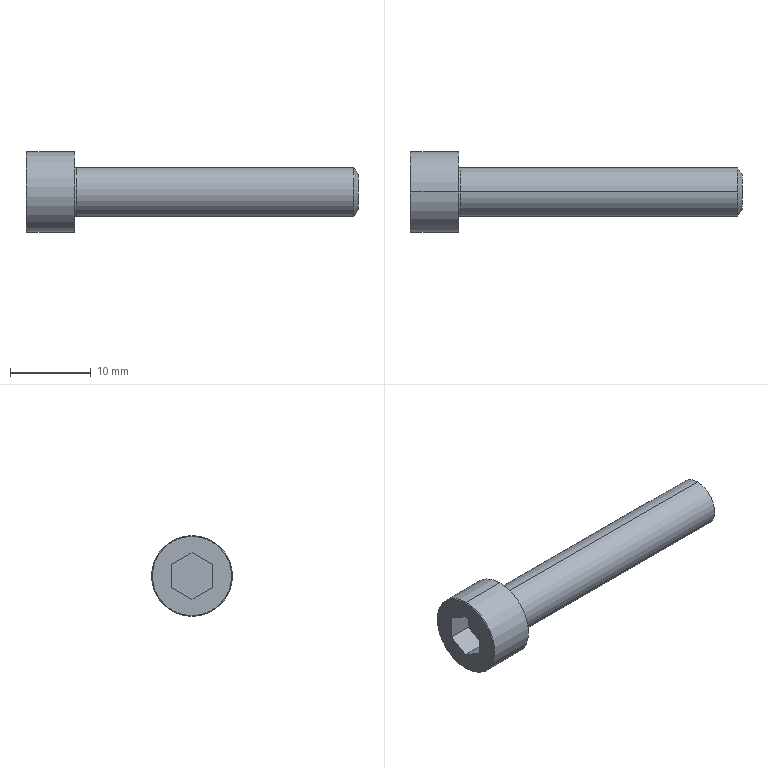Part | SolidWorks | features BlendCut 1, Cut 1, Fillet 1, RevCut 1, Revolution 1 | 1 solid | 20 faces | box 41 x 10 x 10 mm | volume 1393 mm3 | plane 10 | torus 4 | cylinder 4 | cone 2 | commonest cylinder face diameters 6 x2 10 x2
STEP:
#1=CARTESIAN_POINT('',(0.,0.,4.9));
#2=VERTEX_POINT('',#1);
#3=CARTESIAN_POINT('',(0.,0.,-4.9));
#4=VERTEX_POINT('',#3);
#5=CARTESIAN_POINT('',(0.,0.,0.));
#6=DIRECTION('',(-1.,0.,0.));
#7=DIRECTION('',(0.,0.,-1.));
#8=AXIS2_PLACEMENT_3D('',#5,#6,#7);
#9=CIRCLE('',#8,4.9);
#10=EDGE_CURVE('',#2,#4,#9,.T.);
#11=ORIENTED_EDGE('',*,*,#10,.F.);
#12=CARTESIAN_POINT('',(0.1,0.,5.));
#13=VERTEX_POINT('',#12);
#14=CARTESIAN_POINT('',(0.1,0.,4.9));
#15=DIRECTION('',(0.,1.,0.));
#16=DIRECTION('',(0.,0.,1.));
#17=AXIS2_PLACEMENT_3D('',#14,#15,#16);
#18=CIRCLE('',#17,0.1);
#19=EDGE_CURVE('',#2,#13,#18,.T.);
#20=ORIENTED_EDGE('',*,*,#19,.T.);
#21=CARTESIAN_POINT('',(0.1,0.,-5.));
#22=VERTEX_POINT('',#21);
#23=CARTESIAN_POINT('',(0.1,0.,0.));
#24=DIRECTION('',(1.,0.,0.));
#25=DIRECTION('',(0.,0.,-1.));
#26=AXIS2_PLACEMENT_3D('',#23,#24,#25);
#27=CIRCLE('',#26,5.);
#28=EDGE_CURVE('',#22,#13,#27,.T.);
#29=ORIENTED_EDGE('',*,*,#28,.F.);
#30=CARTESIAN_POINT('',(0.1,0.,-4.9));
#31=DIRECTION('',(0.,-1.,0.));
#32=DIRECTION('',(1.,0.,0.));
#33=AXIS2_PLACEMENT_3D('',#30,#31,#32);
#34=CIRCLE('',#33,0.1);
#35=EDGE_CURVE('',#4,#22,#34,.T.);
#36=ORIENTED_EDGE('',*,*,#35,.F.);
#37=EDGE_LOOP('',(#11,#20,#29,#36));
#38=FACE_OUTER_BOUND('',#37,.T.);
#39=CARTESIAN_POINT('',(0.1,0.,0.));
#40=DIRECTION('',(1.,0.,0.));
#41=DIRECTION('',(0.,0.,-1.));
#42=AXIS2_PLACEMENT_3D('',#39,#40,#41);
#43=TOROIDAL_SURFACE('',#42,4.9,0.1);
#44=ADVANCED_FACE('',(#38),#43,.T.);
#45=CARTESIAN_POINT('',(41.,0.,2.134));
#46=VERTEX_POINT('',#45);
#47=CARTESIAN_POINT('',(41.,0.,-2.134));
#48=VERTEX_POINT('',#47);
#49=CARTESIAN_POINT('',(41.,0.,0.));
#50=DIRECTION('',(-1.,0.,0.));
#51=DIRECTION('',(0.,0.,1.));
#52=AXIS2_PLACEMENT_3D('',#49,#50,#51);
#53=CIRCLE('',#52,2.134);
#54=EDGE_CURVE('',#46,#48,#53,.T.);
#55=ORIENTED_EDGE('',*,*,#54,.T.);
#56=CARTESIAN_POINT('',(40.5,0.,-3.));
#57=VERTEX_POINT('',#56);
#58=CARTESIAN_POINT('',(40.5,0.,-3.));
#59=DIRECTION('',(-0.5,0.,-0.866));
#60=VECTOR('',#59,1000.);
#61=LINE('',#58,#60);
#62=EDGE_CURVE('',#48,#57,#61,.T.);
#63=ORIENTED_EDGE('',*,*,#62,.T.);
#64=CARTESIAN_POINT('',(40.5,0.,3.));
#65=VERTEX_POINT('',#64);
#66=CARTESIAN_POINT('',(40.5,0.,0.));
#67=DIRECTION('',(-1.,0.,0.));
#68=DIRECTION('',(0.,0.,1.));
#69=AXIS2_PLACEMENT_3D('',#66,#67,#68);
#70=CIRCLE('',#69,3.);
#71=EDGE_CURVE('',#65,#57,#70,.T.);
#72=ORIENTED_EDGE('',*,*,#71,.F.);
#73=CARTESIAN_POINT('',(40.5,0.,3.));
#74=DIRECTION('',(-0.5,0.,0.866));
#75=VECTOR('',#74,1000.);
#76=LINE('',#73,#75);
#77=EDGE_CURVE('',#46,#65,#76,.T.);
#78=ORIENTED_EDGE('',*,*,#77,.F.);
#79=EDGE_LOOP('',(#55,#63,#72,#78));
#80=FACE_OUTER_BOUND('',#79,.T.);
#81=CARTESIAN_POINT('',(40.5,0.,0.));
#82=DIRECTION('',(-1.,0.,0.));
#83=DIRECTION('',(0.,0.,1.));
#84=AXIS2_PLACEMENT_3D('',#81,#82,#83);
#85=CONICAL_SURFACE('',#84,3.,1.047);
#86=ADVANCED_FACE('',(#80),#85,.T.);
#87=CARTESIAN_POINT('',(6.,0.,-3.2));
#88=VERTEX_POINT('',#87);
#89=CARTESIAN_POINT('',(6.,0.,3.2));
#90=VERTEX_POINT('',#89);
#91=CARTESIAN_POINT('',(6.,0.,0.));
#92=DIRECTION('',(-1.,0.,0.));
#93=DIRECTION('',(0.,0.,1.));
#94=AXIS2_PLACEMENT_3D('',#91,#92,#93);
#95=CIRCLE('',#94,3.2);
#96=EDGE_CURVE('',#88,#90,#95,.T.);
#97=ORIENTED_EDGE('',*,*,#96,.F.);
#98=CARTESIAN_POINT('',(6.2,0.,-3.));
#99=VERTEX_POINT('',#98);
#100=CARTESIAN_POINT('',(6.2,0.,-3.2));
#101=DIRECTION('',(0.,1.,0.));
#102=DIRECTION('',(-1.,0.,0.));
#103=AXIS2_PLACEMENT_3D('',#100,#101,#102);
#104=CIRCLE('',#103,0.2);
#105=EDGE_CURVE('',#88,#99,#104,.T.);
#106=ORIENTED_EDGE('',*,*,#105,.T.);
#107=CARTESIAN_POINT('',(6.2,0.,3.));
#108=VERTEX_POINT('',#107);
#109=CARTESIAN_POINT('',(6.2,0.,0.));
#110=DIRECTION('',(-1.,0.,0.));
#111=DIRECTION('',(0.,0.,1.));
#112=AXIS2_PLACEMENT_3D('',#109,#110,#111);
#113=CIRCLE('',#112,3.);
#114=EDGE_CURVE('',#99,#108,#113,.T.);
#115=ORIENTED_EDGE('',*,*,#114,.T.);
#116=CARTESIAN_POINT('',(6.2,0.,3.2));
#117=DIRECTION('',(0.,-1.,0.));
#118=DIRECTION('',(1.,0.,0.));
#119=AXIS2_PLACEMENT_3D('',#116,#117,#118);
#120=CIRCLE('',#119,0.2);
#121=EDGE_CURVE('',#90,#108,#120,.T.);
#122=ORIENTED_EDGE('',*,*,#121,.F.);
#123=EDGE_LOOP('',(#97,#106,#115,#122));
#124=FACE_OUTER_BOUND('',#123,.T.);
#125=CARTESIAN_POINT('',(6.2,0.,0.));
#126=DIRECTION('',(-1.,0.,0.));
#127=DIRECTION('',(0.,0.,1.));
#128=AXIS2_PLACEMENT_3D('',#125,#126,#127);
#129=TOROIDAL_SURFACE('',#128,3.2,0.2);
#130=ADVANCED_FACE('',(#124),#129,.F.);
#131=CARTESIAN_POINT('',(6.,0.,5.));
#132=VERTEX_POINT('',#131);
#133=CARTESIAN_POINT('',(6.,0.,-5.));
#134=VERTEX_POINT('',#133);
#135=CARTESIAN_POINT('',(6.,0.,0.));
#136=DIRECTION('',(-1.,0.,0.));
#137=DIRECTION('',(0.,0.,1.));
#138=AXIS2_PLACEMENT_3D('',#135,#136,#137);
#139=CIRCLE('',#138,5.);
#140=EDGE_CURVE('',#132,#134,#139,.T.);
#141=ORIENTED_EDGE('',*,*,#140,.T.);
#142=CARTESIAN_POINT('',(0.,0.,-5.));
#143=DIRECTION('',(-1.,0.,0.));
#144=VECTOR('',#143,1000.);
#145=LINE('',#142,#144);
#146=EDGE_CURVE('',#134,#22,#145,.T.);
#147=ORIENTED_EDGE('',*,*,#146,.T.);
#148=ORIENTED_EDGE('',*,*,#28,.T.);
#149=CARTESIAN_POINT('',(0.,0.,5.));
#150=DIRECTION('',(-1.,0.,0.));
#151=VECTOR('',#150,1000.);
#152=LINE('',#149,#151);
#153=EDGE_CURVE('',#132,#13,#152,.T.);
#154=ORIENTED_EDGE('',*,*,#153,.F.);
#155=EDGE_LOOP('',(#141,#147,#148,#154));
#156=FACE_OUTER_BOUND('',#155,.T.);
#157=CARTESIAN_POINT('',(0.,0.,0.));
#158=DIRECTION('',(-1.,0.,0.));
#159=DIRECTION('',(0.,0.,1.));
#160=AXIS2_PLACEMENT_3D('',#157,#158,#159);
#161=CYLINDRICAL_SURFACE('',#160,5.);
#162=ADVANCED_FACE('',(#156),#161,.T.);
#163=ORIENTED_EDGE('',*,*,#71,.T.);
#164=CARTESIAN_POINT('',(0.,0.,-3.));
#165=DIRECTION('',(-1.,0.,0.));
#166=VECTOR('',#165,1000.);
#167=LINE('',#164,#166);
#168=EDGE_CURVE('',#57,#99,#167,.T.);
#169=ORIENTED_EDGE('',*,*,#168,.T.);
#170=CARTESIAN_POINT('',(6.2,0.,0.));
#171=DIRECTION('',(-1.,0.,0.));
#172=DIRECTION('',(0.,0.,1.));
#173=AXIS2_PLACEMENT_3D('',#170,#171,#172);
#174=CIRCLE('',#173,3.);
#175=EDGE_CURVE('',#108,#99,#174,.T.);
#176=ORIENTED_EDGE('',*,*,#175,.F.);
#177=CARTESIAN_POINT('',(0.,0.,3.));
#178=DIRECTION('',(-1.,0.,0.));
#179=VECTOR('',#178,1000.);
#180=LINE('',#177,#179);
#181=EDGE_CURVE('',#65,#108,#180,.T.);
#182=ORIENTED_EDGE('',*,*,#181,.F.);
#183=EDGE_LOOP('',(#163,#169,#176,#182));
#184=FACE_OUTER_BOUND('',#183,.T.);
#185=CARTESIAN_POINT('',(0.,0.,0.));
#186=DIRECTION('',(-1.,0.,0.));
#187=DIRECTION('',(0.,0.,1.));
#188=AXIS2_PLACEMENT_3D('',#185,#186,#187);
#189=CYLINDRICAL_SURFACE('',#188,3.);
#190=ADVANCED_FACE('',(#184),#189,.T.);
#191=ORIENTED_EDGE('',*,*,#168,.F.);
#192=CARTESIAN_POINT('',(40.5,0.,0.));
#193=DIRECTION('',(-1.,0.,0.));
#194=DIRECTION('',(0.,0.,1.));
#195=AXIS2_PLACEMENT_3D('',#192,#193,#194);
#196=CIRCLE('',#195,3.);
#197=EDGE_CURVE('',#57,#65,#196,.T.);
#198=ORIENTED_EDGE('',*,*,#197,.T.);
#199=ORIENTED_EDGE('',*,*,#181,.T.);
#200=ORIENTED_EDGE('',*,*,#114,.F.);
#201=EDGE_LOOP('',(#191,#198,#199,#200));
#202=FACE_OUTER_BOUND('',#201,.T.);
#203=CARTESIAN_POINT('',(0.,0.,0.));
#204=DIRECTION('',(-1.,0.,0.));
#205=DIRECTION('',(0.,0.,1.));
#206=AXIS2_PLACEMENT_3D('',#203,#204,#205);
#207=CYLINDRICAL_SURFACE('',#206,3.);
#208=ADVANCED_FACE('',(#202),#207,.T.);
#209=CARTESIAN_POINT('',(0.,0.,0.));
#210=DIRECTION('',(-1.,0.,0.));
#211=DIRECTION('',(0.,0.,-1.));
#212=AXIS2_PLACEMENT_3D('',#209,#210,#211);
#213=CIRCLE('',#212,4.9);
#214=EDGE_CURVE('',#4,#2,#213,.T.);
#215=ORIENTED_EDGE('',*,*,#214,.T.);
#216=ORIENTED_EDGE('',*,*,#10,.T.);
#217=EDGE_LOOP('',(#215,#216));
#218=FACE_OUTER_BOUND('',#217,.T.);
#219=CARTESIAN_POINT('',(0.,0.,2.86));
#220=VERTEX_POINT('',#219);
#221=CARTESIAN_POINT('',(0.,2.477,1.43));
#222=VERTEX_POINT('',#221);
#223=CARTESIAN_POINT('',(0.,0.,2.86));
#224=DIRECTION('',(0.,0.866,-0.5));
#225=VECTOR('',#224,1000.);
#226=LINE('',#223,#225);
#227=EDGE_CURVE('',#220,#222,#226,.T.);
#228=ORIENTED_EDGE('',*,*,#227,.F.);
#229=CARTESIAN_POINT('',(0.,-2.477,1.43));
#230=VERTEX_POINT('',#229);
#231=CARTESIAN_POINT('',(0.,-2.477,1.43));
#232=DIRECTION('',(0.,0.866,0.5));
#233=VECTOR('',#232,1000.);
#234=LINE('',#231,#233);
#235=EDGE_CURVE('',#230,#220,#234,.T.);
#236=ORIENTED_EDGE('',*,*,#235,.F.);
#237=CARTESIAN_POINT('',(0.,-2.477,-1.43));
#238=VERTEX_POINT('',#237);
#239=CARTESIAN_POINT('',(0.,-2.477,-1.43));
#240=DIRECTION('',(0.,0.,1.));
#241=VECTOR('',#240,1000.);
#242=LINE('',#239,#241);
#243=EDGE_CURVE('',#238,#230,#242,.T.);
#244=ORIENTED_EDGE('',*,*,#243,.F.);
#245=CARTESIAN_POINT('',(0.,0.,-2.86));
#246=VERTEX_POINT('',#245);
#247=CARTESIAN_POINT('',(0.,0.,-2.86));
#248=DIRECTION('',(0.,-0.866,0.5));
#249=VECTOR('',#248,1000.);
#250=LINE('',#247,#249);
#251=EDGE_CURVE('',#246,#238,#250,.T.);
#252=ORIENTED_EDGE('',*,*,#251,.F.);
#253=CARTESIAN_POINT('',(0.,2.477,-1.43));
#254=VERTEX_POINT('',#253);
#255=CARTESIAN_POINT('',(0.,2.477,-1.43));
#256=DIRECTION('',(0.,-0.866,-0.5));
#257=VECTOR('',#256,1000.);
#258=LINE('',#255,#257);
#259=EDGE_CURVE('',#254,#246,#258,.T.);
#260=ORIENTED_EDGE('',*,*,#259,.F.);
#261=CARTESIAN_POINT('',(0.,2.477,1.43));
#262=DIRECTION('',(0.,0.,-1.));
#263=VECTOR('',#262,1000.);
#264=LINE('',#261,#263);
#265=EDGE_CURVE('',#222,#254,#264,.T.);
#266=ORIENTED_EDGE('',*,*,#265,.F.);
#267=EDGE_LOOP('',(#228,#236,#244,#252,#260,#266));
#268=FACE_BOUND('',#267,.T.);
#269=CARTESIAN_POINT('',(0.,0.,0.));
#270=DIRECTION('',(1.,0.,0.));
#271=DIRECTION('',(0.,0.,-1.));
#272=AXIS2_PLACEMENT_3D('',#269,#270,#271);
#273=PLANE('',#272);
#274=ADVANCED_FACE('',(#218,#268),#273,.F.);
#275=ORIENTED_EDGE('',*,*,#146,.F.);
#276=CARTESIAN_POINT('',(6.,0.,0.));
#277=DIRECTION('',(-1.,0.,0.));
#278=DIRECTION('',(0.,0.,1.));
#279=AXIS2_PLACEMENT_3D('',#276,#277,#278);
#280=CIRCLE('',#279,5.);
#281=EDGE_CURVE('',#134,#132,#280,.T.);
#282=ORIENTED_EDGE('',*,*,#281,.T.);
#283=ORIENTED_EDGE('',*,*,#153,.T.);
#284=CARTESIAN_POINT('',(0.1,0.,0.));
#285=DIRECTION('',(1.,0.,0.));
#286=DIRECTION('',(0.,0.,-1.));
#287=AXIS2_PLACEMENT_3D('',#284,#285,#286);
#288=CIRCLE('',#287,5.);
#289=EDGE_CURVE('',#13,#22,#288,.T.);
#290=ORIENTED_EDGE('',*,*,#289,.T.);
#291=EDGE_LOOP('',(#275,#282,#283,#290));
#292=FACE_OUTER_BOUND('',#291,.T.);
#293=CARTESIAN_POINT('',(0.,0.,0.));
#294=DIRECTION('',(-1.,0.,0.));
#295=DIRECTION('',(0.,0.,1.));
#296=AXIS2_PLACEMENT_3D('',#293,#294,#295);
#297=CYLINDRICAL_SURFACE('',#296,5.);
#298=ADVANCED_FACE('',(#292),#297,.T.);
#299=ORIENTED_EDGE('',*,*,#140,.F.);
#300=ORIENTED_EDGE('',*,*,#281,.F.);
#301=EDGE_LOOP('',(#299,#300));
#302=FACE_OUTER_BOUND('',#301,.T.);
#303=CARTESIAN_POINT('',(6.,0.,0.));
#304=DIRECTION('',(-1.,0.,0.));
#305=DIRECTION('',(0.,0.,1.));
#306=AXIS2_PLACEMENT_3D('',#303,#304,#305);
#307=CIRCLE('',#306,3.2);
#308=EDGE_CURVE('',#90,#88,#307,.T.);
#309=ORIENTED_EDGE('',*,*,#308,.T.);
#310=ORIENTED_EDGE('',*,*,#96,.T.);
#311=EDGE_LOOP('',(#309,#310));
#312=FACE_BOUND('',#311,.T.);
#313=CARTESIAN_POINT('',(6.,5.,0.));
#314=DIRECTION('',(-1.,0.,0.));
#315=DIRECTION('',(0.,0.,1.));
#316=AXIS2_PLACEMENT_3D('',#313,#314,#315);
#317=PLANE('',#316);
#318=ADVANCED_FACE('',(#302,#312),#317,.F.);
#319=ORIENTED_EDGE('',*,*,#105,.F.);
#320=ORIENTED_EDGE('',*,*,#308,.F.);
#321=ORIENTED_EDGE('',*,*,#121,.T.);
#322=ORIENTED_EDGE('',*,*,#175,.T.);
#323=EDGE_LOOP('',(#319,#320,#321,#322));
#324=FACE_OUTER_BOUND('',#323,.T.);
#325=CARTESIAN_POINT('',(6.2,0.,0.));
#326=DIRECTION('',(-1.,0.,0.));
#327=DIRECTION('',(0.,0.,1.));
#328=AXIS2_PLACEMENT_3D('',#325,#326,#327);
#329=TOROIDAL_SURFACE('',#328,3.2,0.2);
#330=ADVANCED_FACE('',(#324),#329,.F.);
#331=ORIENTED_EDGE('',*,*,#235,.T.);
#332=CARTESIAN_POINT('',(3.,0.,2.86));
#333=VERTEX_POINT('',#332);
#334=CARTESIAN_POINT('',(3.,0.,2.86));
#335=DIRECTION('',(-1.,0.,0.));
#336=VECTOR('',#335,1000.);
#337=LINE('',#334,#336);
#338=EDGE_CURVE('',#333,#220,#337,.T.);
#339=ORIENTED_EDGE('',*,*,#338,.F.);
#340=CARTESIAN_POINT('',(3.,-2.477,1.43));
#341=VERTEX_POINT('',#340);
#342=CARTESIAN_POINT('',(3.,-2.477,1.43));
#343=DIRECTION('',(0.,0.866,0.5));
#344=VECTOR('',#343,1000.);
#345=LINE('',#342,#344);
#346=EDGE_CURVE('',#341,#333,#345,.T.);
#347=ORIENTED_EDGE('',*,*,#346,.F.);
#348=CARTESIAN_POINT('',(3.,-2.477,1.43));
#349=DIRECTION('',(-1.,0.,0.));
#350=VECTOR('',#349,1000.);
#351=LINE('',#348,#350);
#352=EDGE_CURVE('',#341,#230,#351,.T.);
#353=ORIENTED_EDGE('',*,*,#352,.T.);
#354=EDGE_LOOP('',(#331,#339,#347,#353));
#355=FACE_OUTER_BOUND('',#354,.T.);
#356=CARTESIAN_POINT('',(3.,-2.477,1.43));
#357=DIRECTION('',(0.,-0.5,0.866));
#358=DIRECTION('',(0.,-0.866,-0.5));
#359=AXIS2_PLACEMENT_3D('',#356,#357,#358);
#360=PLANE('',#359);
#361=ADVANCED_FACE('',(#355),#360,.F.);
#362=ORIENTED_EDGE('',*,*,#243,.T.);
#363=ORIENTED_EDGE('',*,*,#352,.F.);
#364=CARTESIAN_POINT('',(3.,-2.477,-1.43));
#365=VERTEX_POINT('',#364);
#366=CARTESIAN_POINT('',(3.,-2.477,-1.43));
#367=DIRECTION('',(0.,0.,1.));
#368=VECTOR('',#367,1000.);
#369=LINE('',#366,#368);
#370=EDGE_CURVE('',#365,#341,#369,.T.);
#371=ORIENTED_EDGE('',*,*,#370,.F.);
#372=CARTESIAN_POINT('',(3.,-2.477,-1.43));
#373=DIRECTION('',(-1.,0.,0.));
#374=VECTOR('',#373,1000.);
#375=LINE('',#372,#374);
#376=EDGE_CURVE('',#365,#238,#375,.T.);
#377=ORIENTED_EDGE('',*,*,#376,.T.);
#378=EDGE_LOOP('',(#362,#363,#371,#377));
#379=FACE_OUTER_BOUND('',#378,.T.);
#380=CARTESIAN_POINT('',(3.,-2.477,-1.43));
#381=DIRECTION('',(0.,-1.,0.));
#382=DIRECTION('',(0.,0.,-1.));
#383=AXIS2_PLACEMENT_3D('',#380,#381,#382);
#384=PLANE('',#383);
#385=ADVANCED_FACE('',(#379),#384,.F.);
#386=ORIENTED_EDGE('',*,*,#251,.T.);
#387=ORIENTED_EDGE('',*,*,#376,.F.);
#388=CARTESIAN_POINT('',(3.,0.,-2.86));
#389=VERTEX_POINT('',#388);
#390=CARTESIAN_POINT('',(3.,0.,-2.86));
#391=DIRECTION('',(0.,-0.866,0.5));
#392=VECTOR('',#391,1000.);
#393=LINE('',#390,#392);
#394=EDGE_CURVE('',#389,#365,#393,.T.);
#395=ORIENTED_EDGE('',*,*,#394,.F.);
#396=CARTESIAN_POINT('',(3.,0.,-2.86));
#397=DIRECTION('',(-1.,0.,0.));
#398=VECTOR('',#397,1000.);
#399=LINE('',#396,#398);
#400=EDGE_CURVE('',#389,#246,#399,.T.);
#401=ORIENTED_EDGE('',*,*,#400,.T.);
#402=EDGE_LOOP('',(#386,#387,#395,#401));
#403=FACE_OUTER_BOUND('',#402,.T.);
#404=CARTESIAN_POINT('',(3.,0.,-2.86));
#405=DIRECTION('',(0.,-0.5,-0.866));
#406=DIRECTION('',(0.,0.866,-0.5));
#407=AXIS2_PLACEMENT_3D('',#404,#405,#406);
#408=PLANE('',#407);
#409=ADVANCED_FACE('',(#403),#408,.F.);
#410=ORIENTED_EDGE('',*,*,#259,.T.);
#411=ORIENTED_EDGE('',*,*,#400,.F.);
#412=CARTESIAN_POINT('',(3.,2.477,-1.43));
#413=VERTEX_POINT('',#412);
#414=CARTESIAN_POINT('',(3.,2.477,-1.43));
#415=DIRECTION('',(0.,-0.866,-0.5));
#416=VECTOR('',#415,1000.);
#417=LINE('',#414,#416);
#418=EDGE_CURVE('',#413,#389,#417,.T.);
#419=ORIENTED_EDGE('',*,*,#418,.F.);
#420=CARTESIAN_POINT('',(3.,2.477,-1.43));
#421=DIRECTION('',(-1.,0.,0.));
#422=VECTOR('',#421,1000.);
#423=LINE('',#420,#422);
#424=EDGE_CURVE('',#413,#254,#423,.T.);
#425=ORIENTED_EDGE('',*,*,#424,.T.);
#426=EDGE_LOOP('',(#410,#411,#419,#425));
#427=FACE_OUTER_BOUND('',#426,.T.);
#428=CARTESIAN_POINT('',(3.,2.477,-1.43));
#429=DIRECTION('',(0.,0.5,-0.866));
#430=DIRECTION('',(0.,0.866,0.5));
#431=AXIS2_PLACEMENT_3D('',#428,#429,#430);
#432=PLANE('',#431);
#433=ADVANCED_FACE('',(#427),#432,.F.);
#434=ORIENTED_EDGE('',*,*,#265,.T.);
#435=ORIENTED_EDGE('',*,*,#424,.F.);
#436=CARTESIAN_POINT('',(3.,2.477,1.43));
#437=VERTEX_POINT('',#436);
#438=CARTESIAN_POINT('',(3.,2.477,1.43));
#439=DIRECTION('',(0.,0.,-1.));
#440=VECTOR('',#439,1000.);
#441=LINE('',#438,#440);
#442=EDGE_CURVE('',#437,#413,#441,.T.);
#443=ORIENTED_EDGE('',*,*,#442,.F.);
#444=CARTESIAN_POINT('',(3.,2.477,1.43));
#445=DIRECTION('',(-1.,0.,0.));
#446=VECTOR('',#445,1000.);
#447=LINE('',#444,#446);
#448=EDGE_CURVE('',#437,#222,#447,.T.);
#449=ORIENTED_EDGE('',*,*,#448,.T.);
#450=EDGE_LOOP('',(#434,#435,#443,#449));
#451=FACE_OUTER_BOUND('',#450,.T.);
#452=CARTESIAN_POINT('',(3.,2.477,1.43));
#453=DIRECTION('',(0.,1.,0.));
#454=DIRECTION('',(0.,0.,1.));
#455=AXIS2_PLACEMENT_3D('',#452,#453,#454);
#456=PLANE('',#455);
#457=ADVANCED_FACE('',(#451),#456,.F.);
#458=ORIENTED_EDGE('',*,*,#227,.T.);
#459=ORIENTED_EDGE('',*,*,#448,.F.);
#460=CARTESIAN_POINT('',(3.,0.,2.86));
#461=DIRECTION('',(0.,0.866,-0.5));
#462=VECTOR('',#461,1000.);
#463=LINE('',#460,#462);
#464=EDGE_CURVE('',#333,#437,#463,.T.);
#465=ORIENTED_EDGE('',*,*,#464,.F.);
#466=ORIENTED_EDGE('',*,*,#338,.T.);
#467=EDGE_LOOP('',(#458,#459,#465,#466));
#468=FACE_OUTER_BOUND('',#467,.T.);
#469=CARTESIAN_POINT('',(3.,0.,2.86));
#470=DIRECTION('',(0.,0.5,0.866));
#471=DIRECTION('',(0.,-0.866,0.5));
#472=AXIS2_PLACEMENT_3D('',#469,#470,#471);
#473=PLANE('',#472);
#474=ADVANCED_FACE('',(#468),#473,.F.);
#475=ORIENTED_EDGE('',*,*,#346,.T.);
#476=ORIENTED_EDGE('',*,*,#464,.T.);
#477=ORIENTED_EDGE('',*,*,#442,.T.);
#478=ORIENTED_EDGE('',*,*,#418,.T.);
#479=ORIENTED_EDGE('',*,*,#394,.T.);
#480=ORIENTED_EDGE('',*,*,#370,.T.);
#481=EDGE_LOOP('',(#475,#476,#477,#478,#479,#480));
#482=FACE_OUTER_BOUND('',#481,.T.);
#483=CARTESIAN_POINT('',(3.,-2.477,1.43));
#484=DIRECTION('',(1.,0.,0.));
#485=DIRECTION('',(0.,0.,-1.));
#486=AXIS2_PLACEMENT_3D('',#483,#484,#485);
#487=PLANE('',#486);
#488=ADVANCED_FACE('',(#482),#487,.F.);
#489=ORIENTED_EDGE('',*,*,#62,.F.);
#490=CARTESIAN_POINT('',(41.,0.,0.));
#491=DIRECTION('',(-1.,0.,0.));
#492=DIRECTION('',(0.,0.,1.));
#493=AXIS2_PLACEMENT_3D('',#490,#491,#492);
#494=CIRCLE('',#493,2.134);
#495=EDGE_CURVE('',#48,#46,#494,.T.);
#496=ORIENTED_EDGE('',*,*,#495,.T.);
#497=ORIENTED_EDGE('',*,*,#77,.T.);
#498=ORIENTED_EDGE('',*,*,#197,.F.);
#499=EDGE_LOOP('',(#489,#496,#497,#498));
#500=FACE_OUTER_BOUND('',#499,.T.);
#501=CARTESIAN_POINT('',(40.5,0.,0.));
#502=DIRECTION('',(-1.,0.,0.));
#503=DIRECTION('',(0.,0.,1.));
#504=AXIS2_PLACEMENT_3D('',#501,#502,#503);
#505=CONICAL_SURFACE('',#504,3.,1.047);
#506=ADVANCED_FACE('',(#500),#505,.T.);
#507=ORIENTED_EDGE('',*,*,#54,.F.);
#508=ORIENTED_EDGE('',*,*,#495,.F.);
#509=EDGE_LOOP('',(#507,#508));
#510=FACE_OUTER_BOUND('',#509,.T.);
#511=CARTESIAN_POINT('',(41.,3.,0.));
#512=DIRECTION('',(-1.,0.,0.));
#513=DIRECTION('',(0.,0.,1.));
#514=AXIS2_PLACEMENT_3D('',#511,#512,#513);
#515=PLANE('',#514);
#516=ADVANCED_FACE('',(#510),#515,.F.);
#517=ORIENTED_EDGE('',*,*,#19,.F.);
#518=ORIENTED_EDGE('',*,*,#214,.F.);
#519=ORIENTED_EDGE('',*,*,#35,.T.);
#520=ORIENTED_EDGE('',*,*,#289,.F.);
#521=EDGE_LOOP('',(#517,#518,#519,#520));
#522=FACE_OUTER_BOUND('',#521,.T.);
#523=CARTESIAN_POINT('',(0.1,0.,0.));
#524=DIRECTION('',(1.,0.,0.));
#525=DIRECTION('',(0.,0.,-1.));
#526=AXIS2_PLACEMENT_3D('',#523,#524,#525);
#527=TOROIDAL_SURFACE('',#526,4.9,0.1);
#528=ADVANCED_FACE('',(#522),#527,.T.);
#529=CLOSED_SHELL('',(#44,#86,#130,#162,#190,#208,#274,#298,#318,#330,#361,#385,#409,#433,#457,#474,#488,#506,#516,#528));
#530=MANIFOLD_SOLID_BREP('',#529);
#531=CARTESIAN_POINT('',(0.,0.,0.));
#532=DIRECTION('',(0.,0.,1.));
#533=DIRECTION('',(1.,0.,0.));
#534=AXIS2_PLACEMENT_3D('',#531,#532,#533);
#535=(LENGTH_UNIT()NAMED_UNIT(*)SI_UNIT(.MILLI.,.METRE.));
#536=UNCERTAINTY_MEASURE_WITH_UNIT(LENGTH_MEASURE(0.00001),#535,'','');
#537=(NAMED_UNIT(*)PLANE_ANGLE_UNIT()SI_UNIT($,.RADIAN.));
#538=(NAMED_UNIT(*)SI_UNIT($,.STERADIAN.)SOLID_ANGLE_UNIT());
#539=(GEOMETRIC_REPRESENTATION_CONTEXT(3)GLOBAL_UNCERTAINTY_ASSIGNED_CONTEXT((#536))GLOBAL_UNIT_ASSIGNED_CONTEXT((#535,#537,#538))REPRESENTATION_CONTEXT('',''));
#540=ADVANCED_BREP_SHAPE_REPRESENTATION('',(#530,#534),#539);